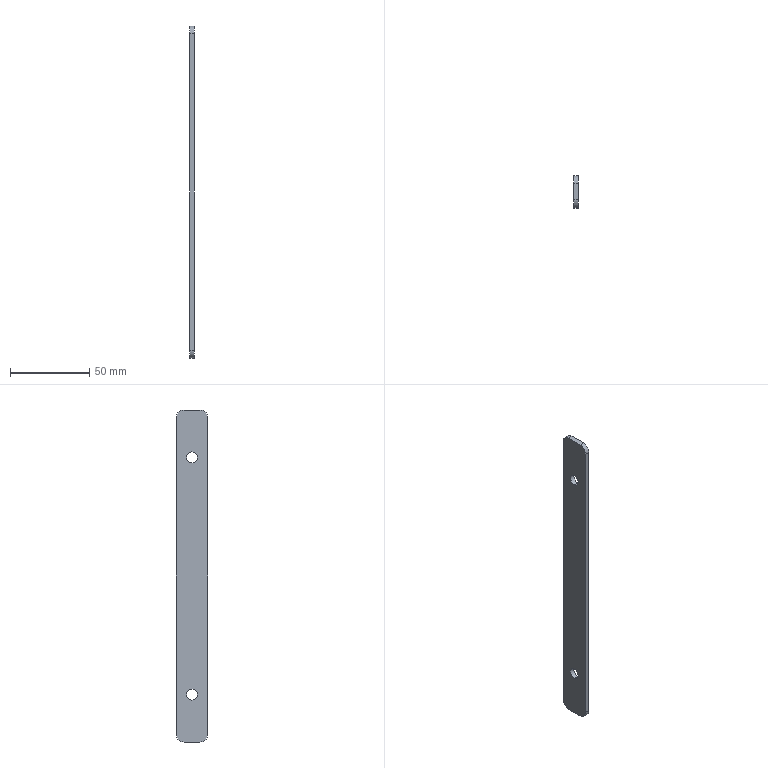Part | SolidWorks | features Fillet 1, FlatPattern 1, HoleWzd 1, SMBaseFlange 1, SheetMetal 1 | 1 solid | 14 faces | box 3 x 20 x 210 mm | volume 12305 mm3 | cylinder 8 | plane 6 | commonest cylinder face diameters 7 x4 10 x4
STEP:
#1=CARTESIAN_POINT('',(-3.,10.,-33.5));
#2=VERTEX_POINT('',#1);
#3=CARTESIAN_POINT('',(-3.,10.,-26.5));
#4=VERTEX_POINT('',#3);
#5=CARTESIAN_POINT('',(-3.,10.,-30.));
#6=DIRECTION('',(-1.,0.,0.));
#7=DIRECTION('',(0.,0.,1.));
#8=AXIS2_PLACEMENT_3D('',#5,#6,#7);
#9=CIRCLE('',#8,3.5);
#10=EDGE_CURVE('',#2,#4,#9,.T.);
#11=ORIENTED_EDGE('',*,*,#10,.T.);
#12=CARTESIAN_POINT('',(0.,10.,-26.5));
#13=VERTEX_POINT('',#12);
#14=CARTESIAN_POINT('',(0.,10.,-26.5));
#15=DIRECTION('',(1.,0.,0.));
#16=VECTOR('',#15,1000.);
#17=LINE('',#14,#16);
#18=EDGE_CURVE('',#4,#13,#17,.T.);
#19=ORIENTED_EDGE('',*,*,#18,.T.);
#20=CARTESIAN_POINT('',(0.,10.,-33.5));
#21=VERTEX_POINT('',#20);
#22=CARTESIAN_POINT('',(0.,10.,-30.));
#23=DIRECTION('',(1.,0.,0.));
#24=DIRECTION('',(0.,0.,-1.));
#25=AXIS2_PLACEMENT_3D('',#22,#23,#24);
#26=CIRCLE('',#25,3.5);
#27=EDGE_CURVE('',#13,#21,#26,.T.);
#28=ORIENTED_EDGE('',*,*,#27,.T.);
#29=CARTESIAN_POINT('',(0.,10.,-33.5));
#30=DIRECTION('',(1.,0.,0.));
#31=VECTOR('',#30,1000.);
#32=LINE('',#29,#31);
#33=EDGE_CURVE('',#2,#21,#32,.T.);
#34=ORIENTED_EDGE('',*,*,#33,.F.);
#35=EDGE_LOOP('',(#11,#19,#28,#34));
#36=FACE_OUTER_BOUND('',#35,.T.);
#37=CARTESIAN_POINT('',(0.,10.,-30.));
#38=DIRECTION('',(1.,0.,0.));
#39=DIRECTION('',(0.,0.,-1.));
#40=AXIS2_PLACEMENT_3D('',#37,#38,#39);
#41=CYLINDRICAL_SURFACE('',#40,3.5);
#42=ADVANCED_FACE('',(#36),#41,.F.);
#43=CARTESIAN_POINT('',(-3.,10.,-183.5));
#44=VERTEX_POINT('',#43);
#45=CARTESIAN_POINT('',(-3.,10.,-176.5));
#46=VERTEX_POINT('',#45);
#47=CARTESIAN_POINT('',(-3.,10.,-180.));
#48=DIRECTION('',(-1.,0.,0.));
#49=DIRECTION('',(0.,0.,1.));
#50=AXIS2_PLACEMENT_3D('',#47,#48,#49);
#51=CIRCLE('',#50,3.5);
#52=EDGE_CURVE('',#44,#46,#51,.T.);
#53=ORIENTED_EDGE('',*,*,#52,.T.);
#54=CARTESIAN_POINT('',(0.,10.,-176.5));
#55=VERTEX_POINT('',#54);
#56=CARTESIAN_POINT('',(0.,10.,-176.5));
#57=DIRECTION('',(1.,0.,0.));
#58=VECTOR('',#57,1000.);
#59=LINE('',#56,#58);
#60=EDGE_CURVE('',#46,#55,#59,.T.);
#61=ORIENTED_EDGE('',*,*,#60,.T.);
#62=CARTESIAN_POINT('',(0.,10.,-183.5));
#63=VERTEX_POINT('',#62);
#64=CARTESIAN_POINT('',(0.,10.,-180.));
#65=DIRECTION('',(1.,0.,0.));
#66=DIRECTION('',(0.,0.,-1.));
#67=AXIS2_PLACEMENT_3D('',#64,#65,#66);
#68=CIRCLE('',#67,3.5);
#69=EDGE_CURVE('',#55,#63,#68,.T.);
#70=ORIENTED_EDGE('',*,*,#69,.T.);
#71=CARTESIAN_POINT('',(0.,10.,-183.5));
#72=DIRECTION('',(1.,0.,0.));
#73=VECTOR('',#72,1000.);
#74=LINE('',#71,#73);
#75=EDGE_CURVE('',#44,#63,#74,.T.);
#76=ORIENTED_EDGE('',*,*,#75,.F.);
#77=EDGE_LOOP('',(#53,#61,#70,#76));
#78=FACE_OUTER_BOUND('',#77,.T.);
#79=CARTESIAN_POINT('',(0.,10.,-180.));
#80=DIRECTION('',(1.,0.,0.));
#81=DIRECTION('',(0.,0.,-1.));
#82=AXIS2_PLACEMENT_3D('',#79,#80,#81);
#83=CYLINDRICAL_SURFACE('',#82,3.5);
#84=ADVANCED_FACE('',(#78),#83,.F.);
#85=CARTESIAN_POINT('',(-3.,15.,0.));
#86=VERTEX_POINT('',#85);
#87=CARTESIAN_POINT('',(-3.,5.,0.));
#88=VERTEX_POINT('',#87);
#89=CARTESIAN_POINT('',(-3.,0.,0.));
#90=DIRECTION('',(0.,-1.,0.));
#91=VECTOR('',#90,1000.);
#92=LINE('',#89,#91);
#93=EDGE_CURVE('',#86,#88,#92,.T.);
#94=ORIENTED_EDGE('',*,*,#93,.T.);
#95=CARTESIAN_POINT('',(0.,5.,0.));
#96=VERTEX_POINT('',#95);
#97=CARTESIAN_POINT('',(-3.,5.,0.));
#98=DIRECTION('',(1.,0.,0.));
#99=VECTOR('',#98,1000.);
#100=LINE('',#97,#99);
#101=EDGE_CURVE('',#88,#96,#100,.T.);
#102=ORIENTED_EDGE('',*,*,#101,.T.);
#103=CARTESIAN_POINT('',(0.,15.,0.));
#104=VERTEX_POINT('',#103);
#105=CARTESIAN_POINT('',(0.,0.,0.));
#106=DIRECTION('',(0.,-1.,0.));
#107=VECTOR('',#106,1000.);
#108=LINE('',#105,#107);
#109=EDGE_CURVE('',#104,#96,#108,.T.);
#110=ORIENTED_EDGE('',*,*,#109,.F.);
#111=CARTESIAN_POINT('',(-3.,15.,0.));
#112=DIRECTION('',(-1.,0.,0.));
#113=VECTOR('',#112,1000.);
#114=LINE('',#111,#113);
#115=EDGE_CURVE('',#104,#86,#114,.T.);
#116=ORIENTED_EDGE('',*,*,#115,.T.);
#117=EDGE_LOOP('',(#94,#102,#110,#116));
#118=FACE_OUTER_BOUND('',#117,.T.);
#119=CARTESIAN_POINT('',(-3.,0.,0.));
#120=DIRECTION('',(0.,0.,1.));
#121=DIRECTION('',(1.,0.,0.));
#122=AXIS2_PLACEMENT_3D('',#119,#120,#121);
#123=PLANE('',#122);
#124=ADVANCED_FACE('',(#118),#123,.T.);
#125=CARTESIAN_POINT('',(0.,20.,-205.));
#126=VERTEX_POINT('',#125);
#127=CARTESIAN_POINT('',(0.,20.,-5.));
#128=VERTEX_POINT('',#127);
#129=CARTESIAN_POINT('',(0.,20.,0.));
#130=DIRECTION('',(0.,0.,1.));
#131=VECTOR('',#130,1000.);
#132=LINE('',#129,#131);
#133=EDGE_CURVE('',#126,#128,#132,.T.);
#134=ORIENTED_EDGE('',*,*,#133,.F.);
#135=CARTESIAN_POINT('',(-3.,20.,-205.));
#136=VERTEX_POINT('',#135);
#137=CARTESIAN_POINT('',(-3.,20.,-205.));
#138=DIRECTION('',(-1.,0.,0.));
#139=VECTOR('',#138,1000.);
#140=LINE('',#137,#139);
#141=EDGE_CURVE('',#126,#136,#140,.T.);
#142=ORIENTED_EDGE('',*,*,#141,.T.);
#143=CARTESIAN_POINT('',(-3.,20.,-5.));
#144=VERTEX_POINT('',#143);
#145=CARTESIAN_POINT('',(-3.,20.,0.));
#146=DIRECTION('',(0.,0.,1.));
#147=VECTOR('',#146,1000.);
#148=LINE('',#145,#147);
#149=EDGE_CURVE('',#136,#144,#148,.T.);
#150=ORIENTED_EDGE('',*,*,#149,.T.);
#151=CARTESIAN_POINT('',(-3.,20.,-5.));
#152=DIRECTION('',(1.,0.,0.));
#153=VECTOR('',#152,1000.);
#154=LINE('',#151,#153);
#155=EDGE_CURVE('',#144,#128,#154,.T.);
#156=ORIENTED_EDGE('',*,*,#155,.T.);
#157=EDGE_LOOP('',(#134,#142,#150,#156));
#158=FACE_OUTER_BOUND('',#157,.T.);
#159=CARTESIAN_POINT('',(-3.,20.,0.));
#160=DIRECTION('',(0.,1.,0.));
#161=DIRECTION('',(0.,0.,1.));
#162=AXIS2_PLACEMENT_3D('',#159,#160,#161);
#163=PLANE('',#162);
#164=ADVANCED_FACE('',(#158),#163,.T.);
#165=CARTESIAN_POINT('',(0.,5.,-210.));
#166=VERTEX_POINT('',#165);
#167=CARTESIAN_POINT('',(0.,15.,-210.));
#168=VERTEX_POINT('',#167);
#169=CARTESIAN_POINT('',(0.,20.,-210.));
#170=DIRECTION('',(0.,1.,0.));
#171=VECTOR('',#170,1000.);
#172=LINE('',#169,#171);
#173=EDGE_CURVE('',#166,#168,#172,.T.);
#174=ORIENTED_EDGE('',*,*,#173,.F.);
#175=CARTESIAN_POINT('',(-3.,5.,-210.));
#176=VERTEX_POINT('',#175);
#177=CARTESIAN_POINT('',(-3.,5.,-210.));
#178=DIRECTION('',(-1.,0.,0.));
#179=VECTOR('',#178,1000.);
#180=LINE('',#177,#179);
#181=EDGE_CURVE('',#166,#176,#180,.T.);
#182=ORIENTED_EDGE('',*,*,#181,.T.);
#183=CARTESIAN_POINT('',(-3.,15.,-210.));
#184=VERTEX_POINT('',#183);
#185=CARTESIAN_POINT('',(-3.,20.,-210.));
#186=DIRECTION('',(0.,1.,0.));
#187=VECTOR('',#186,1000.);
#188=LINE('',#185,#187);
#189=EDGE_CURVE('',#176,#184,#188,.T.);
#190=ORIENTED_EDGE('',*,*,#189,.T.);
#191=CARTESIAN_POINT('',(-3.,15.,-210.));
#192=DIRECTION('',(1.,0.,0.));
#193=VECTOR('',#192,1000.);
#194=LINE('',#191,#193);
#195=EDGE_CURVE('',#184,#168,#194,.T.);
#196=ORIENTED_EDGE('',*,*,#195,.T.);
#197=EDGE_LOOP('',(#174,#182,#190,#196));
#198=FACE_OUTER_BOUND('',#197,.T.);
#199=CARTESIAN_POINT('',(-3.,20.,-210.));
#200=DIRECTION('',(0.,0.,-1.));
#201=DIRECTION('',(-1.,0.,0.));
#202=AXIS2_PLACEMENT_3D('',#199,#200,#201);
#203=PLANE('',#202);
#204=ADVANCED_FACE('',(#198),#203,.T.);
#205=CARTESIAN_POINT('',(-3.,0.,-5.));
#206=VERTEX_POINT('',#205);
#207=CARTESIAN_POINT('',(-3.,0.,-205.));
#208=VERTEX_POINT('',#207);
#209=CARTESIAN_POINT('',(-3.,0.,0.));
#210=DIRECTION('',(0.,0.,-1.));
#211=VECTOR('',#210,1000.);
#212=LINE('',#209,#211);
#213=EDGE_CURVE('',#206,#208,#212,.T.);
#214=ORIENTED_EDGE('',*,*,#213,.T.);
#215=CARTESIAN_POINT('',(0.,0.,-205.));
#216=VERTEX_POINT('',#215);
#217=CARTESIAN_POINT('',(-3.,0.,-205.));
#218=DIRECTION('',(1.,0.,0.));
#219=VECTOR('',#218,1000.);
#220=LINE('',#217,#219);
#221=EDGE_CURVE('',#208,#216,#220,.T.);
#222=ORIENTED_EDGE('',*,*,#221,.T.);
#223=CARTESIAN_POINT('',(0.,0.,-5.));
#224=VERTEX_POINT('',#223);
#225=CARTESIAN_POINT('',(0.,0.,0.));
#226=DIRECTION('',(0.,0.,-1.));
#227=VECTOR('',#226,1000.);
#228=LINE('',#225,#227);
#229=EDGE_CURVE('',#224,#216,#228,.T.);
#230=ORIENTED_EDGE('',*,*,#229,.F.);
#231=CARTESIAN_POINT('',(-3.,0.,-5.));
#232=DIRECTION('',(-1.,0.,0.));
#233=VECTOR('',#232,1000.);
#234=LINE('',#231,#233);
#235=EDGE_CURVE('',#224,#206,#234,.T.);
#236=ORIENTED_EDGE('',*,*,#235,.T.);
#237=EDGE_LOOP('',(#214,#222,#230,#236));
#238=FACE_OUTER_BOUND('',#237,.T.);
#239=CARTESIAN_POINT('',(-3.,0.,0.));
#240=DIRECTION('',(0.,-1.,0.));
#241=DIRECTION('',(0.,0.,-1.));
#242=AXIS2_PLACEMENT_3D('',#239,#240,#241);
#243=PLANE('',#242);
#244=ADVANCED_FACE('',(#238),#243,.T.);
#245=ORIENTED_EDGE('',*,*,#10,.F.);
#246=CARTESIAN_POINT('',(-3.,10.,-30.));
#247=DIRECTION('',(-1.,0.,0.));
#248=DIRECTION('',(0.,0.,1.));
#249=AXIS2_PLACEMENT_3D('',#246,#247,#248);
#250=CIRCLE('',#249,3.5);
#251=EDGE_CURVE('',#4,#2,#250,.T.);
#252=ORIENTED_EDGE('',*,*,#251,.F.);
#253=EDGE_LOOP('',(#245,#252));
#254=FACE_BOUND('',#253,.T.);
#255=ORIENTED_EDGE('',*,*,#52,.F.);
#256=CARTESIAN_POINT('',(-3.,10.,-180.));
#257=DIRECTION('',(-1.,0.,0.));
#258=DIRECTION('',(0.,0.,1.));
#259=AXIS2_PLACEMENT_3D('',#256,#257,#258);
#260=CIRCLE('',#259,3.5);
#261=EDGE_CURVE('',#46,#44,#260,.T.);
#262=ORIENTED_EDGE('',*,*,#261,.F.);
#263=EDGE_LOOP('',(#255,#262));
#264=FACE_BOUND('',#263,.T.);
#265=ORIENTED_EDGE('',*,*,#189,.F.);
#266=CARTESIAN_POINT('',(-3.,5.,-205.));
#267=DIRECTION('',(-1.,0.,0.));
#268=DIRECTION('',(0.,0.,1.));
#269=AXIS2_PLACEMENT_3D('',#266,#267,#268);
#270=CIRCLE('',#269,5.);
#271=EDGE_CURVE('',#176,#208,#270,.T.);
#272=ORIENTED_EDGE('',*,*,#271,.T.);
#273=ORIENTED_EDGE('',*,*,#213,.F.);
#274=CARTESIAN_POINT('',(-3.,5.,-5.));
#275=DIRECTION('',(-1.,0.,0.));
#276=DIRECTION('',(0.,0.,1.));
#277=AXIS2_PLACEMENT_3D('',#274,#275,#276);
#278=CIRCLE('',#277,5.);
#279=EDGE_CURVE('',#206,#88,#278,.T.);
#280=ORIENTED_EDGE('',*,*,#279,.T.);
#281=ORIENTED_EDGE('',*,*,#93,.F.);
#282=CARTESIAN_POINT('',(-3.,15.,-5.));
#283=DIRECTION('',(-1.,0.,0.));
#284=DIRECTION('',(0.,0.,1.));
#285=AXIS2_PLACEMENT_3D('',#282,#283,#284);
#286=CIRCLE('',#285,5.);
#287=EDGE_CURVE('',#86,#144,#286,.T.);
#288=ORIENTED_EDGE('',*,*,#287,.T.);
#289=ORIENTED_EDGE('',*,*,#149,.F.);
#290=CARTESIAN_POINT('',(-3.,15.,-205.));
#291=DIRECTION('',(-1.,0.,0.));
#292=DIRECTION('',(0.,0.,1.));
#293=AXIS2_PLACEMENT_3D('',#290,#291,#292);
#294=CIRCLE('',#293,5.);
#295=EDGE_CURVE('',#136,#184,#294,.T.);
#296=ORIENTED_EDGE('',*,*,#295,.T.);
#297=EDGE_LOOP('',(#265,#272,#273,#280,#281,#288,#289,#296));
#298=FACE_OUTER_BOUND('',#297,.T.);
#299=CARTESIAN_POINT('',(-3.,0.,0.));
#300=DIRECTION('',(-1.,0.,0.));
#301=DIRECTION('',(0.,0.,1.));
#302=AXIS2_PLACEMENT_3D('',#299,#300,#301);
#303=PLANE('',#302);
#304=ADVANCED_FACE('',(#254,#264,#298),#303,.T.);
#305=CARTESIAN_POINT('',(0.,10.,-30.));
#306=DIRECTION('',(1.,0.,0.));
#307=DIRECTION('',(0.,0.,-1.));
#308=AXIS2_PLACEMENT_3D('',#305,#306,#307);
#309=CIRCLE('',#308,3.5);
#310=EDGE_CURVE('',#21,#13,#309,.T.);
#311=ORIENTED_EDGE('',*,*,#310,.F.);
#312=ORIENTED_EDGE('',*,*,#27,.F.);
#313=EDGE_LOOP('',(#311,#312));
#314=FACE_BOUND('',#313,.T.);
#315=CARTESIAN_POINT('',(0.,10.,-180.));
#316=DIRECTION('',(1.,0.,0.));
#317=DIRECTION('',(0.,0.,-1.));
#318=AXIS2_PLACEMENT_3D('',#315,#316,#317);
#319=CIRCLE('',#318,3.5);
#320=EDGE_CURVE('',#63,#55,#319,.T.);
#321=ORIENTED_EDGE('',*,*,#320,.F.);
#322=ORIENTED_EDGE('',*,*,#69,.F.);
#323=EDGE_LOOP('',(#321,#322));
#324=FACE_BOUND('',#323,.T.);
#325=ORIENTED_EDGE('',*,*,#229,.T.);
#326=CARTESIAN_POINT('',(0.,5.,-205.));
#327=DIRECTION('',(1.,0.,0.));
#328=DIRECTION('',(0.,0.,1.));
#329=AXIS2_PLACEMENT_3D('',#326,#327,#328);
#330=CIRCLE('',#329,5.);
#331=EDGE_CURVE('',#216,#166,#330,.T.);
#332=ORIENTED_EDGE('',*,*,#331,.T.);
#333=ORIENTED_EDGE('',*,*,#173,.T.);
#334=CARTESIAN_POINT('',(0.,15.,-205.));
#335=DIRECTION('',(1.,0.,0.));
#336=DIRECTION('',(0.,0.,1.));
#337=AXIS2_PLACEMENT_3D('',#334,#335,#336);
#338=CIRCLE('',#337,5.);
#339=EDGE_CURVE('',#168,#126,#338,.T.);
#340=ORIENTED_EDGE('',*,*,#339,.T.);
#341=ORIENTED_EDGE('',*,*,#133,.T.);
#342=CARTESIAN_POINT('',(0.,15.,-5.));
#343=DIRECTION('',(1.,0.,0.));
#344=DIRECTION('',(0.,0.,1.));
#345=AXIS2_PLACEMENT_3D('',#342,#343,#344);
#346=CIRCLE('',#345,5.);
#347=EDGE_CURVE('',#128,#104,#346,.T.);
#348=ORIENTED_EDGE('',*,*,#347,.T.);
#349=ORIENTED_EDGE('',*,*,#109,.T.);
#350=CARTESIAN_POINT('',(0.,5.,-5.));
#351=DIRECTION('',(1.,0.,0.));
#352=DIRECTION('',(0.,0.,1.));
#353=AXIS2_PLACEMENT_3D('',#350,#351,#352);
#354=CIRCLE('',#353,5.);
#355=EDGE_CURVE('',#96,#224,#354,.T.);
#356=ORIENTED_EDGE('',*,*,#355,.T.);
#357=EDGE_LOOP('',(#325,#332,#333,#340,#341,#348,#349,#356));
#358=FACE_OUTER_BOUND('',#357,.T.);
#359=CARTESIAN_POINT('',(0.,0.,0.));
#360=DIRECTION('',(-1.,0.,0.));
#361=DIRECTION('',(0.,0.,1.));
#362=AXIS2_PLACEMENT_3D('',#359,#360,#361);
#363=PLANE('',#362);
#364=ADVANCED_FACE('',(#314,#324,#358),#363,.F.);
#365=ORIENTED_EDGE('',*,*,#60,.F.);
#366=ORIENTED_EDGE('',*,*,#261,.T.);
#367=ORIENTED_EDGE('',*,*,#75,.T.);
#368=ORIENTED_EDGE('',*,*,#320,.T.);
#369=EDGE_LOOP('',(#365,#366,#367,#368));
#370=FACE_OUTER_BOUND('',#369,.T.);
#371=CARTESIAN_POINT('',(0.,10.,-180.));
#372=DIRECTION('',(1.,0.,0.));
#373=DIRECTION('',(0.,0.,-1.));
#374=AXIS2_PLACEMENT_3D('',#371,#372,#373);
#375=CYLINDRICAL_SURFACE('',#374,3.5);
#376=ADVANCED_FACE('',(#370),#375,.F.);
#377=ORIENTED_EDGE('',*,*,#18,.F.);
#378=ORIENTED_EDGE('',*,*,#251,.T.);
#379=ORIENTED_EDGE('',*,*,#33,.T.);
#380=ORIENTED_EDGE('',*,*,#310,.T.);
#381=EDGE_LOOP('',(#377,#378,#379,#380));
#382=FACE_OUTER_BOUND('',#381,.T.);
#383=CARTESIAN_POINT('',(0.,10.,-30.));
#384=DIRECTION('',(1.,0.,0.));
#385=DIRECTION('',(0.,0.,-1.));
#386=AXIS2_PLACEMENT_3D('',#383,#384,#385);
#387=CYLINDRICAL_SURFACE('',#386,3.5);
#388=ADVANCED_FACE('',(#382),#387,.F.);
#389=ORIENTED_EDGE('',*,*,#271,.F.);
#390=ORIENTED_EDGE('',*,*,#181,.F.);
#391=ORIENTED_EDGE('',*,*,#331,.F.);
#392=ORIENTED_EDGE('',*,*,#221,.F.);
#393=EDGE_LOOP('',(#389,#390,#391,#392));
#394=FACE_OUTER_BOUND('',#393,.T.);
#395=CARTESIAN_POINT('',(-3.,5.,-205.));
#396=DIRECTION('',(1.,0.,0.));
#397=DIRECTION('',(0.,0.,-1.));
#398=AXIS2_PLACEMENT_3D('',#395,#396,#397);
#399=CYLINDRICAL_SURFACE('',#398,5.);
#400=ADVANCED_FACE('',(#394),#399,.T.);
#401=ORIENTED_EDGE('',*,*,#295,.F.);
#402=ORIENTED_EDGE('',*,*,#141,.F.);
#403=ORIENTED_EDGE('',*,*,#339,.F.);
#404=ORIENTED_EDGE('',*,*,#195,.F.);
#405=EDGE_LOOP('',(#401,#402,#403,#404));
#406=FACE_OUTER_BOUND('',#405,.T.);
#407=CARTESIAN_POINT('',(-3.,15.,-205.));
#408=DIRECTION('',(1.,0.,0.));
#409=DIRECTION('',(0.,0.,-1.));
#410=AXIS2_PLACEMENT_3D('',#407,#408,#409);
#411=CYLINDRICAL_SURFACE('',#410,5.);
#412=ADVANCED_FACE('',(#406),#411,.T.);
#413=ORIENTED_EDGE('',*,*,#279,.F.);
#414=ORIENTED_EDGE('',*,*,#235,.F.);
#415=ORIENTED_EDGE('',*,*,#355,.F.);
#416=ORIENTED_EDGE('',*,*,#101,.F.);
#417=EDGE_LOOP('',(#413,#414,#415,#416));
#418=FACE_OUTER_BOUND('',#417,.T.);
#419=CARTESIAN_POINT('',(-3.,5.,-5.));
#420=DIRECTION('',(1.,0.,0.));
#421=DIRECTION('',(0.,0.,-1.));
#422=AXIS2_PLACEMENT_3D('',#419,#420,#421);
#423=CYLINDRICAL_SURFACE('',#422,5.);
#424=ADVANCED_FACE('',(#418),#423,.T.);
#425=ORIENTED_EDGE('',*,*,#287,.F.);
#426=ORIENTED_EDGE('',*,*,#115,.F.);
#427=ORIENTED_EDGE('',*,*,#347,.F.);
#428=ORIENTED_EDGE('',*,*,#155,.F.);
#429=EDGE_LOOP('',(#425,#426,#427,#428));
#430=FACE_OUTER_BOUND('',#429,.T.);
#431=CARTESIAN_POINT('',(-3.,15.,-5.));
#432=DIRECTION('',(1.,0.,0.));
#433=DIRECTION('',(0.,0.,-1.));
#434=AXIS2_PLACEMENT_3D('',#431,#432,#433);
#435=CYLINDRICAL_SURFACE('',#434,5.);
#436=ADVANCED_FACE('',(#430),#435,.T.);
#437=CLOSED_SHELL('',(#42,#84,#124,#164,#204,#244,#304,#364,#376,#388,#400,#412,#424,#436));
#438=MANIFOLD_SOLID_BREP('',#437);
#439=CARTESIAN_POINT('',(0.,0.,0.));
#440=DIRECTION('',(0.,0.,1.));
#441=DIRECTION('',(1.,0.,0.));
#442=AXIS2_PLACEMENT_3D('',#439,#440,#441);
#443=(LENGTH_UNIT()NAMED_UNIT(*)SI_UNIT(.MILLI.,.METRE.));
#444=UNCERTAINTY_MEASURE_WITH_UNIT(LENGTH_MEASURE(0.00001),#443,'','');
#445=(NAMED_UNIT(*)PLANE_ANGLE_UNIT()SI_UNIT($,.RADIAN.));
#446=(NAMED_UNIT(*)SI_UNIT($,.STERADIAN.)SOLID_ANGLE_UNIT());
#447=(GEOMETRIC_REPRESENTATION_CONTEXT(3)GLOBAL_UNCERTAINTY_ASSIGNED_CONTEXT((#444))GLOBAL_UNIT_ASSIGNED_CONTEXT((#443,#445,#446))REPRESENTATION_CONTEXT('',''));
#448=ADVANCED_BREP_SHAPE_REPRESENTATION('',(#438,#442),#447);